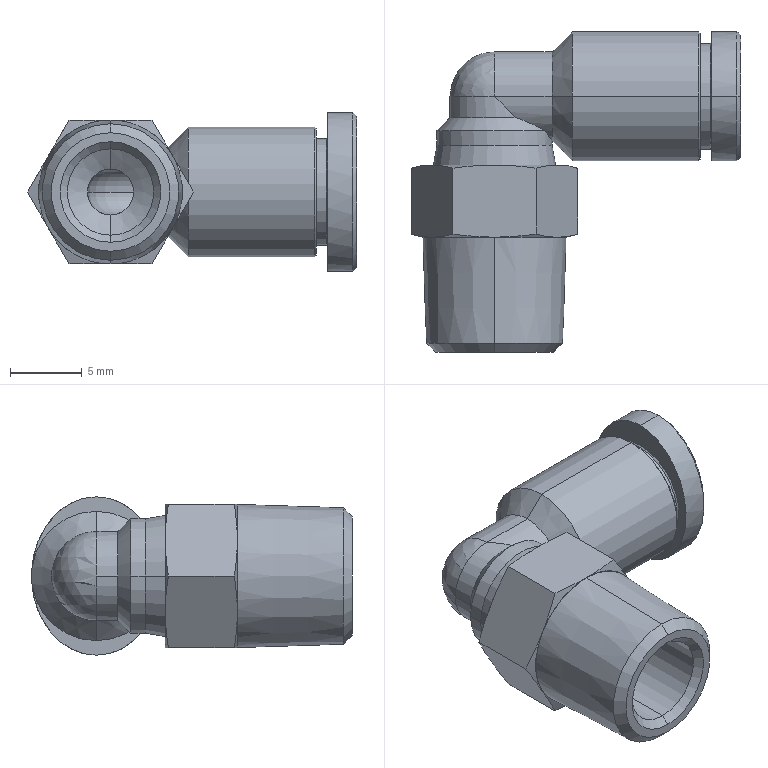Part | STEP file | L-type fitting PL4-01 | 1 solid | 66 faces | box 22.874 x 22.3 x 11 mm | volume 1653 mm3 | cone 29 | cylinder 17 | plane 13 | spline 4 | torus 2 | sphere 1 | commonest cylinder face diameters 6.2 x5 3.2 x2 4 x2 6 x2 7.4 x2 8 x2